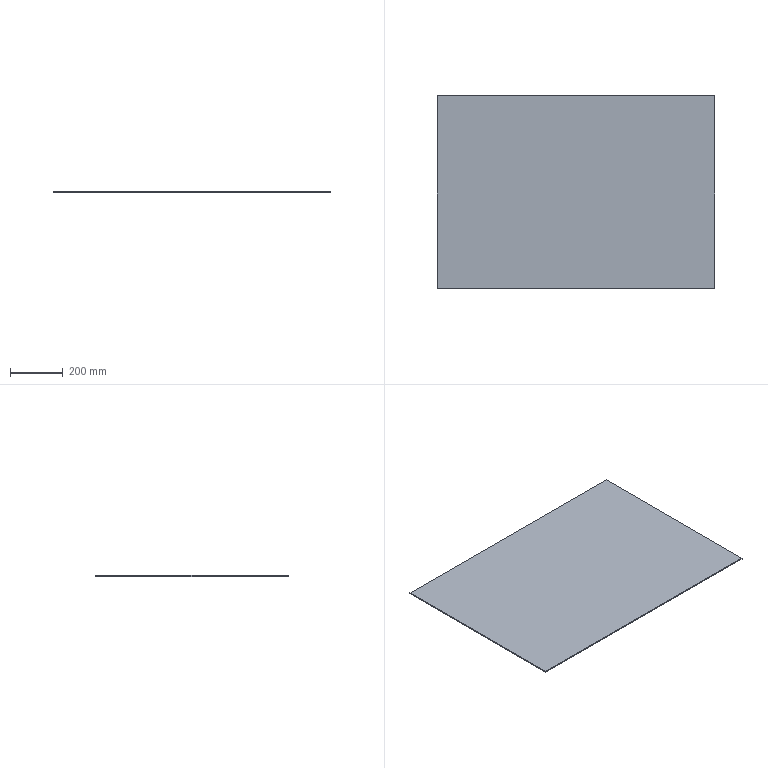Part | SolidWorks | features Extrusion 1 | 1 solid | 6 faces | box 1048 x 726 x 4 mm | volume 3043392 mm3 | plane 6
STEP:
#1=CARTESIAN_POINT('',(-524.,363.,0.));
#2=VERTEX_POINT('',#1);
#3=CARTESIAN_POINT('',(-524.,-363.,0.));
#4=VERTEX_POINT('',#3);
#5=CARTESIAN_POINT('',(-524.,-363.,0.));
#6=DIRECTION('',(0.,-1.,0.));
#7=VECTOR('',#6,1000.);
#8=LINE('',#5,#7);
#9=EDGE_CURVE('',#2,#4,#8,.T.);
#10=ORIENTED_EDGE('',*,*,#9,.T.);
#11=CARTESIAN_POINT('',(-524.,-363.,4.));
#12=VERTEX_POINT('',#11);
#13=CARTESIAN_POINT('',(-524.,-363.,4.));
#14=DIRECTION('',(0.,0.,-1.));
#15=VECTOR('',#14,1000.);
#16=LINE('',#13,#15);
#17=EDGE_CURVE('',#12,#4,#16,.T.);
#18=ORIENTED_EDGE('',*,*,#17,.F.);
#19=CARTESIAN_POINT('',(-524.,363.,4.));
#20=VERTEX_POINT('',#19);
#21=CARTESIAN_POINT('',(-524.,-363.,4.));
#22=DIRECTION('',(0.,-1.,0.));
#23=VECTOR('',#22,1000.);
#24=LINE('',#21,#23);
#25=EDGE_CURVE('',#20,#12,#24,.T.);
#26=ORIENTED_EDGE('',*,*,#25,.F.);
#27=CARTESIAN_POINT('',(-524.,363.,4.));
#28=DIRECTION('',(0.,0.,-1.));
#29=VECTOR('',#28,1000.);
#30=LINE('',#27,#29);
#31=EDGE_CURVE('',#20,#2,#30,.T.);
#32=ORIENTED_EDGE('',*,*,#31,.T.);
#33=EDGE_LOOP('',(#10,#18,#26,#32));
#34=FACE_OUTER_BOUND('',#33,.T.);
#35=CARTESIAN_POINT('',(-524.,-363.,4.));
#36=DIRECTION('',(1.,0.,0.));
#37=DIRECTION('',(0.,0.,-1.));
#38=AXIS2_PLACEMENT_3D('',#35,#36,#37);
#39=PLANE('',#38);
#40=ADVANCED_FACE('',(#34),#39,.F.);
#41=CARTESIAN_POINT('',(524.,-363.,0.));
#42=VERTEX_POINT('',#41);
#43=CARTESIAN_POINT('',(524.,-363.,0.));
#44=DIRECTION('',(1.,0.,0.));
#45=VECTOR('',#44,1000.);
#46=LINE('',#43,#45);
#47=EDGE_CURVE('',#4,#42,#46,.T.);
#48=ORIENTED_EDGE('',*,*,#47,.T.);
#49=CARTESIAN_POINT('',(524.,-363.,4.));
#50=VERTEX_POINT('',#49);
#51=CARTESIAN_POINT('',(524.,-363.,4.));
#52=DIRECTION('',(0.,0.,-1.));
#53=VECTOR('',#52,1000.);
#54=LINE('',#51,#53);
#55=EDGE_CURVE('',#50,#42,#54,.T.);
#56=ORIENTED_EDGE('',*,*,#55,.F.);
#57=CARTESIAN_POINT('',(524.,-363.,4.));
#58=DIRECTION('',(1.,0.,0.));
#59=VECTOR('',#58,1000.);
#60=LINE('',#57,#59);
#61=EDGE_CURVE('',#12,#50,#60,.T.);
#62=ORIENTED_EDGE('',*,*,#61,.F.);
#63=ORIENTED_EDGE('',*,*,#17,.T.);
#64=EDGE_LOOP('',(#48,#56,#62,#63));
#65=FACE_OUTER_BOUND('',#64,.T.);
#66=CARTESIAN_POINT('',(524.,-363.,4.));
#67=DIRECTION('',(0.,1.,0.));
#68=DIRECTION('',(-1.,0.,0.));
#69=AXIS2_PLACEMENT_3D('',#66,#67,#68);
#70=PLANE('',#69);
#71=ADVANCED_FACE('',(#65),#70,.F.);
#72=CARTESIAN_POINT('',(524.,363.,0.));
#73=VERTEX_POINT('',#72);
#74=CARTESIAN_POINT('',(524.,-363.,0.));
#75=DIRECTION('',(0.,1.,0.));
#76=VECTOR('',#75,1000.);
#77=LINE('',#74,#76);
#78=EDGE_CURVE('',#42,#73,#77,.T.);
#79=ORIENTED_EDGE('',*,*,#78,.T.);
#80=CARTESIAN_POINT('',(524.,363.,4.));
#81=VERTEX_POINT('',#80);
#82=CARTESIAN_POINT('',(524.,363.,4.));
#83=DIRECTION('',(0.,0.,-1.));
#84=VECTOR('',#83,1000.);
#85=LINE('',#82,#84);
#86=EDGE_CURVE('',#81,#73,#85,.T.);
#87=ORIENTED_EDGE('',*,*,#86,.F.);
#88=CARTESIAN_POINT('',(524.,-363.,4.));
#89=DIRECTION('',(0.,1.,0.));
#90=VECTOR('',#89,1000.);
#91=LINE('',#88,#90);
#92=EDGE_CURVE('',#50,#81,#91,.T.);
#93=ORIENTED_EDGE('',*,*,#92,.F.);
#94=ORIENTED_EDGE('',*,*,#55,.T.);
#95=EDGE_LOOP('',(#79,#87,#93,#94));
#96=FACE_OUTER_BOUND('',#95,.T.);
#97=CARTESIAN_POINT('',(524.,-363.,4.));
#98=DIRECTION('',(-1.,0.,0.));
#99=DIRECTION('',(0.,0.,1.));
#100=AXIS2_PLACEMENT_3D('',#97,#98,#99);
#101=PLANE('',#100);
#102=ADVANCED_FACE('',(#96),#101,.F.);
#103=CARTESIAN_POINT('',(524.,363.,0.));
#104=DIRECTION('',(-1.,0.,0.));
#105=VECTOR('',#104,1000.);
#106=LINE('',#103,#105);
#107=EDGE_CURVE('',#73,#2,#106,.T.);
#108=ORIENTED_EDGE('',*,*,#107,.T.);
#109=ORIENTED_EDGE('',*,*,#31,.F.);
#110=CARTESIAN_POINT('',(524.,363.,4.));
#111=DIRECTION('',(-1.,0.,0.));
#112=VECTOR('',#111,1000.);
#113=LINE('',#110,#112);
#114=EDGE_CURVE('',#81,#20,#113,.T.);
#115=ORIENTED_EDGE('',*,*,#114,.F.);
#116=ORIENTED_EDGE('',*,*,#86,.T.);
#117=EDGE_LOOP('',(#108,#109,#115,#116));
#118=FACE_OUTER_BOUND('',#117,.T.);
#119=CARTESIAN_POINT('',(524.,363.,4.));
#120=DIRECTION('',(0.,-1.,0.));
#121=DIRECTION('',(1.,0.,0.));
#122=AXIS2_PLACEMENT_3D('',#119,#120,#121);
#123=PLANE('',#122);
#124=ADVANCED_FACE('',(#118),#123,.F.);
#125=ORIENTED_EDGE('',*,*,#25,.T.);
#126=ORIENTED_EDGE('',*,*,#61,.T.);
#127=ORIENTED_EDGE('',*,*,#92,.T.);
#128=ORIENTED_EDGE('',*,*,#114,.T.);
#129=EDGE_LOOP('',(#125,#126,#127,#128));
#130=FACE_OUTER_BOUND('',#129,.T.);
#131=CARTESIAN_POINT('',(0.,0.,4.));
#132=DIRECTION('',(0.,0.,1.));
#133=DIRECTION('',(1.,0.,0.));
#134=AXIS2_PLACEMENT_3D('',#131,#132,#133);
#135=PLANE('',#134);
#136=ADVANCED_FACE('',(#130),#135,.T.);
#137=ORIENTED_EDGE('',*,*,#9,.F.);
#138=ORIENTED_EDGE('',*,*,#107,.F.);
#139=ORIENTED_EDGE('',*,*,#78,.F.);
#140=ORIENTED_EDGE('',*,*,#47,.F.);
#141=EDGE_LOOP('',(#137,#138,#139,#140));
#142=FACE_OUTER_BOUND('',#141,.T.);
#143=CARTESIAN_POINT('',(0.,0.,0.));
#144=DIRECTION('',(0.,0.,1.));
#145=DIRECTION('',(1.,0.,0.));
#146=AXIS2_PLACEMENT_3D('',#143,#144,#145);
#147=PLANE('',#146);
#148=ADVANCED_FACE('',(#142),#147,.F.);
#149=CLOSED_SHELL('',(#40,#71,#102,#124,#136,#148));
#150=MANIFOLD_SOLID_BREP('',#149);
#151=CARTESIAN_POINT('',(0.,0.,0.));
#152=DIRECTION('',(0.,0.,1.));
#153=DIRECTION('',(1.,0.,0.));
#154=AXIS2_PLACEMENT_3D('',#151,#152,#153);
#155=(LENGTH_UNIT()NAMED_UNIT(*)SI_UNIT(.MILLI.,.METRE.));
#156=UNCERTAINTY_MEASURE_WITH_UNIT(LENGTH_MEASURE(0.00001),#155,'','');
#157=(NAMED_UNIT(*)PLANE_ANGLE_UNIT()SI_UNIT($,.RADIAN.));
#158=(NAMED_UNIT(*)SI_UNIT($,.STERADIAN.)SOLID_ANGLE_UNIT());
#159=(GEOMETRIC_REPRESENTATION_CONTEXT(3)GLOBAL_UNCERTAINTY_ASSIGNED_CONTEXT((#156))GLOBAL_UNIT_ASSIGNED_CONTEXT((#155,#157,#158))REPRESENTATION_CONTEXT('',''));
#160=ADVANCED_BREP_SHAPE_REPRESENTATION('',(#150,#154),#159);